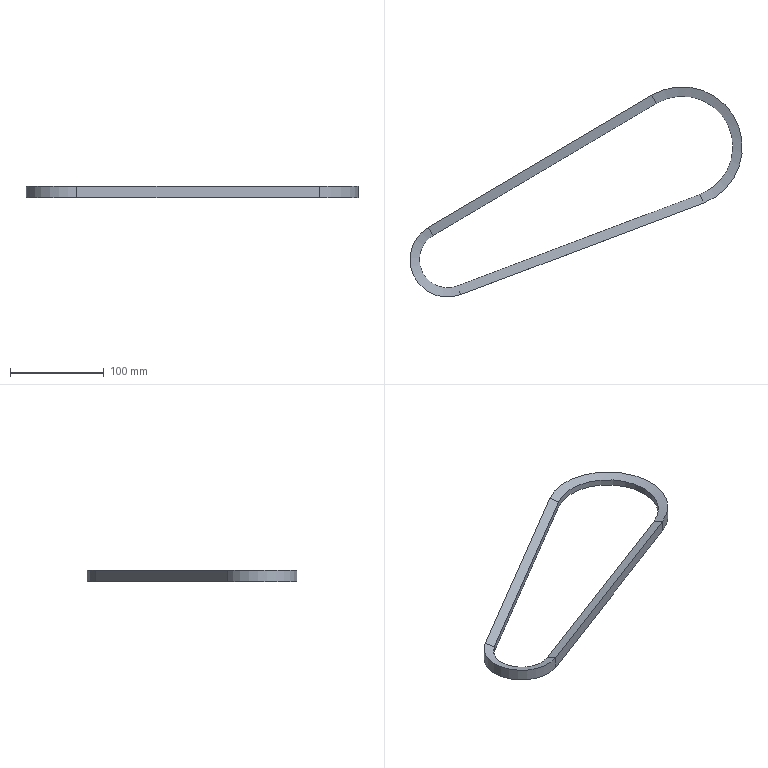Part | STEP file | Type A V-belt | 1 solid | 16 faces | box 354 x 224 x 12.68 mm | volume 82452 mm3 | plane 8 | cylinder 4 | cone 4 | commonest cylinder face diameters 60 x1 80 x1 108 x1 128 x1
STEP:
#1=CARTESIAN_POINT('',(0.,0.,0.));
#2=DIRECTION('',(0.,0.,1.));
#3=DIRECTION('',(1.,0.,0.));
#4=AXIS2_PLACEMENT_3D('',#1,#2,#3);
#5=CARTESIAN_POINT('',(10.593,-28.068,3.3));
#6=VERTEX_POINT('',#5);
#7=CARTESIAN_POINT('',(-15.274,25.821,3.3));
#8=VERTEX_POINT('',#7);
#9=CARTESIAN_POINT('',(0.,0.,3.3));
#10=DIRECTION('',(0.,0.,-1.));
#11=DIRECTION('',(-1.,0.,0.));
#12=AXIS2_PLACEMENT_3D('',#9,#10,#11);
#13=CIRCLE('',#12,30.);
#14=CARTESIAN_POINT('',(0.,0.,0.));
#15=DIRECTION('',(0.,0.,-1.));
#16=DIRECTION('',(-1.,0.,0.));
#17=AXIS2_PLACEMENT_3D('',#14,#15,#16);
#18=CYLINDRICAL_SURFACE('',#17,30.);
#19=CARTESIAN_POINT('',(0.,-3.3));
#20=DIRECTION('',(1.,0.));
#21=VECTOR('',#20,1.);
#22=LINE('',#19,#21);
#23=(GEOMETRIC_REPRESENTATION_CONTEXT(2)PARAMETRIC_REPRESENTATION_CONTEXT()REPRESENTATION_CONTEXT('',''));
#24=DEFINITIONAL_REPRESENTATION('',(#22),#23);
#25=PCURVE('',#18,#24);
#26=CARTESIAN_POINT('',(0.,0.,6.34));
#27=DIRECTION('',(0.,0.,1.));
#28=DIRECTION('',(1.,0.,0.));
#29=AXIS2_PLACEMENT_3D('',#26,#27,#28);
#30=CONICAL_SURFACE('',#29,40.,1.276);
#31=CARTESIAN_POINT('',(9.425,-3.04));
#32=DIRECTION('',(-1.,0.));
#33=VECTOR('',#32,1.);
#34=LINE('',#31,#33);
#35=(GEOMETRIC_REPRESENTATION_CONTEXT(2)PARAMETRIC_REPRESENTATION_CONTEXT()REPRESENTATION_CONTEXT('',''));
#36=DEFINITIONAL_REPRESENTATION('',(#34),#35);
#37=PCURVE('',#30,#36);
#38=SURFACE_CURVE('',#13,(#25,#37),.PCURVE_S1.);
#39=EDGE_CURVE('',#6,#8,#38,.T.);
#40=ORIENTED_EDGE('',*,*,#39,.T.);
#41=CARTESIAN_POINT('',(-15.274,25.821,-3.3));
#42=VERTEX_POINT('',#41);
#43=CARTESIAN_POINT('',(-15.274,25.821,3.3));
#44=CARTESIAN_POINT('',(-15.274,25.821,1.1));
#45=CARTESIAN_POINT('',(-15.274,25.821,-1.1));
#46=CARTESIAN_POINT('',(-15.274,25.821,-3.3));
#47=B_SPLINE_CURVE_WITH_KNOTS('',3,(#43,#44,#45,#46),.UNSPECIFIED.,.F.,.F.,(4,4),(0.,1.),.PIECEWISE_BEZIER_KNOTS.);
#48=CARTESIAN_POINT('',(7.32,-3.3));
#49=CARTESIAN_POINT('',(7.32,3.3));
#50=B_SPLINE_CURVE_WITH_KNOTS('',1,(#48,#49),.UNSPECIFIED.,.F.,.F.,(2,2),(0.,1.),.PIECEWISE_BEZIER_KNOTS.);
#51=(GEOMETRIC_REPRESENTATION_CONTEXT(2)PARAMETRIC_REPRESENTATION_CONTEXT()REPRESENTATION_CONTEXT('',''));
#52=DEFINITIONAL_REPRESENTATION('',(#50),#51);
#53=PCURVE('',#18,#52);
#54=CARTESIAN_POINT('',(222.507,166.477,-3.3));
#55=DIRECTION('',(-0.5091,0.8607,0.));
#56=DIRECTION('',(-0.8607,-0.5091,0.));
#57=AXIS2_PLACEMENT_3D('',#54,#55,#56);
#58=PLANE('',#57);
#59=CARTESIAN_POINT('',(276.268,6.6));
#60=CARTESIAN_POINT('',(276.268,4.4));
#61=CARTESIAN_POINT('',(276.268,2.2));
#62=CARTESIAN_POINT('',(276.268,0.));
#63=B_SPLINE_CURVE_WITH_KNOTS('',3,(#59,#60,#61,#62),.UNSPECIFIED.,.F.,.F.,(4,4),(0.,1.),.PIECEWISE_BEZIER_KNOTS.);
#64=(GEOMETRIC_REPRESENTATION_CONTEXT(2)PARAMETRIC_REPRESENTATION_CONTEXT()REPRESENTATION_CONTEXT('',''));
#65=DEFINITIONAL_REPRESENTATION('',(#63),#64);
#66=PCURVE('',#58,#65);
#67=SURFACE_CURVE('',#47,(#53,#66),.PCURVE_S1.);
#68=EDGE_CURVE('',#8,#42,#67,.T.);
#69=ORIENTED_EDGE('',*,*,#68,.T.);
#70=CARTESIAN_POINT('',(10.593,-28.068,-3.3));
#71=VERTEX_POINT('',#70);
#72=CARTESIAN_POINT('',(0.,0.,-3.3));
#73=DIRECTION('',(0.,0.,-1.));
#74=DIRECTION('',(-1.,0.,0.));
#75=AXIS2_PLACEMENT_3D('',#72,#73,#74);
#76=CIRCLE('',#75,30.);
#77=CARTESIAN_POINT('',(0.,3.3));
#78=DIRECTION('',(1.,0.));
#79=VECTOR('',#78,1.);
#80=LINE('',#77,#79);
#81=(GEOMETRIC_REPRESENTATION_CONTEXT(2)PARAMETRIC_REPRESENTATION_CONTEXT()REPRESENTATION_CONTEXT('',''));
#82=DEFINITIONAL_REPRESENTATION('',(#80),#81);
#83=PCURVE('',#18,#82);
#84=CARTESIAN_POINT('',(0.,0.,-3.3));
#85=DIRECTION('',(0.,0.,-1.));
#86=DIRECTION('',(-1.,0.,0.));
#87=AXIS2_PLACEMENT_3D('',#84,#85,#86);
#88=CONICAL_SURFACE('',#87,30.,1.276);
#89=CARTESIAN_POINT('',(0.,0.));
#90=DIRECTION('',(1.,0.));
#91=VECTOR('',#90,1.);
#92=LINE('',#89,#91);
#93=(GEOMETRIC_REPRESENTATION_CONTEXT(2)PARAMETRIC_REPRESENTATION_CONTEXT()REPRESENTATION_CONTEXT('',''));
#94=DEFINITIONAL_REPRESENTATION('',(#92),#93);
#95=PCURVE('',#88,#94);
#96=SURFACE_CURVE('',#76,(#83,#95),.PCURVE_S1.);
#97=EDGE_CURVE('',#71,#42,#96,.T.);
#98=ORIENTED_EDGE('',*,*,#97,.F.);
#99=CARTESIAN_POINT('',(10.593,-28.068,-3.3));
#100=DIRECTION('',(0.,0.,-1.));
#101=VECTOR('',#100,1.);
#102=LINE('',#99,#101);
#103=CARTESIAN_POINT('',(4.352,3.3));
#104=DIRECTION('',(0.,1.));
#105=VECTOR('',#104,1.);
#106=LINE('',#103,#105);
#107=(GEOMETRIC_REPRESENTATION_CONTEXT(2)PARAMETRIC_REPRESENTATION_CONTEXT()REPRESENTATION_CONTEXT('',''));
#108=DEFINITIONAL_REPRESENTATION('',(#106),#107);
#109=PCURVE('',#18,#108);
#110=CARTESIAN_POINT('',(269.067,69.478,-3.3));
#111=DIRECTION('',(-0.3531,0.9356,0.));
#112=DIRECTION('',(-0.9356,-0.3531,0.));
#113=AXIS2_PLACEMENT_3D('',#110,#111,#112);
#114=PLANE('',#113);
#115=CARTESIAN_POINT('',(276.268,0.));
#116=DIRECTION('',(0.,-1.));
#117=VECTOR('',#116,1.);
#118=LINE('',#115,#117);
#119=(GEOMETRIC_REPRESENTATION_CONTEXT(2)PARAMETRIC_REPRESENTATION_CONTEXT()REPRESENTATION_CONTEXT('',''));
#120=DEFINITIONAL_REPRESENTATION('',(#118),#119);
#121=PCURVE('',#114,#120);
#122=SURFACE_CURVE('',#102,(#109,#121),.PCURVE_S1.);
#123=EDGE_CURVE('',#6,#71,#122,.T.);
#124=ORIENTED_EDGE('',*,*,#123,.F.);
#125=EDGE_LOOP('',(#40,#69,#98,#124));
#126=FACE_BOUND('',#125,.F.);
#127=ADVANCED_FACE('',(#126),#18,.F.);
#128=ORIENTED_EDGE('',*,*,#97,.T.);
#129=CARTESIAN_POINT('',(-20.365,34.428,-6.34));
#130=VERTEX_POINT('',#129);
#131=CARTESIAN_POINT('',(-15.274,25.821,-3.3));
#132=CARTESIAN_POINT('',(-16.971,28.69,-4.313));
#133=CARTESIAN_POINT('',(-18.668,31.559,-5.327));
#134=CARTESIAN_POINT('',(-20.365,34.428,-6.34));
#135=B_SPLINE_CURVE_WITH_KNOTS('',3,(#131,#132,#133,#134),.UNSPECIFIED.,.F.,.F.,(4,4),(0.,1.),.PIECEWISE_BEZIER_KNOTS.);
#136=CARTESIAN_POINT('',(7.32,0.));
#137=CARTESIAN_POINT('',(7.32,3.04));
#138=B_SPLINE_CURVE_WITH_KNOTS('',1,(#136,#137),.UNSPECIFIED.,.F.,.F.,(2,2),(0.,1.),.PIECEWISE_BEZIER_KNOTS.);
#139=(GEOMETRIC_REPRESENTATION_CONTEXT(2)PARAMETRIC_REPRESENTATION_CONTEXT()REPRESENTATION_CONTEXT('',''));
#140=DEFINITIONAL_REPRESENTATION('',(#138),#139);
#141=PCURVE('',#88,#140);
#142=CARTESIAN_POINT('',(217.416,175.084,-6.34));
#143=DIRECTION('',(-0.1481,0.2503,0.9568));
#144=DIRECTION('',(0.,-0.9674,0.2531));
#145=AXIS2_PLACEMENT_3D('',#142,#143,#144);
#146=PLANE('',#145);
#147=CARTESIAN_POINT('',(145.172,-235.284));
#148=CARTESIAN_POINT('',(142.14,-237.));
#149=CARTESIAN_POINT('',(139.108,-238.716));
#150=CARTESIAN_POINT('',(136.076,-240.432));
#151=B_SPLINE_CURVE_WITH_KNOTS('',3,(#147,#148,#149,#150),.UNSPECIFIED.,.F.,.F.,(4,4),(0.,1.),.PIECEWISE_BEZIER_KNOTS.);
#152=(GEOMETRIC_REPRESENTATION_CONTEXT(2)PARAMETRIC_REPRESENTATION_CONTEXT()REPRESENTATION_CONTEXT('',''));
#153=DEFINITIONAL_REPRESENTATION('',(#151),#152);
#154=PCURVE('',#146,#153);
#155=SURFACE_CURVE('',#135,(#141,#154),.PCURVE_S1.);
#156=EDGE_CURVE('',#42,#130,#155,.T.);
#157=ORIENTED_EDGE('',*,*,#156,.T.);
#158=CARTESIAN_POINT('',(14.123,-37.424,-6.34));
#159=VERTEX_POINT('',#158);
#160=CARTESIAN_POINT('',(0.,0.,-6.34));
#161=DIRECTION('',(0.,0.,-1.));
#162=DIRECTION('',(-1.,0.,0.));
#163=AXIS2_PLACEMENT_3D('',#160,#161,#162);
#164=CIRCLE('',#163,40.);
#165=CARTESIAN_POINT('',(0.,3.04));
#166=DIRECTION('',(1.,0.));
#167=VECTOR('',#166,1.);
#168=LINE('',#165,#167);
#169=(GEOMETRIC_REPRESENTATION_CONTEXT(2)PARAMETRIC_REPRESENTATION_CONTEXT()REPRESENTATION_CONTEXT('',''));
#170=DEFINITIONAL_REPRESENTATION('',(#168),#169);
#171=PCURVE('',#88,#170);
#172=CARTESIAN_POINT('',(0.,0.,0.));
#173=DIRECTION('',(0.,0.,-1.));
#174=DIRECTION('',(-1.,0.,0.));
#175=AXIS2_PLACEMENT_3D('',#172,#173,#174);
#176=CYLINDRICAL_SURFACE('',#175,40.);
#177=CARTESIAN_POINT('',(0.,6.34));
#178=DIRECTION('',(1.,0.));
#179=VECTOR('',#178,1.);
#180=LINE('',#177,#179);
#181=(GEOMETRIC_REPRESENTATION_CONTEXT(2)PARAMETRIC_REPRESENTATION_CONTEXT()REPRESENTATION_CONTEXT('',''));
#182=DEFINITIONAL_REPRESENTATION('',(#180),#181);
#183=PCURVE('',#176,#182);
#184=SURFACE_CURVE('',#164,(#171,#183),.PCURVE_S1.);
#185=EDGE_CURVE('',#159,#130,#184,.T.);
#186=ORIENTED_EDGE('',*,*,#185,.F.);
#187=CARTESIAN_POINT('',(14.123,-37.424,-6.34));
#188=DIRECTION('',(0.3378,-0.8951,-0.2909));
#189=VECTOR('',#188,1.);
#190=LINE('',#187,#189);
#191=CARTESIAN_POINT('',(4.352,3.04));
#192=DIRECTION('',(0.,1.));
#193=VECTOR('',#192,1.);
#194=LINE('',#191,#193);
#195=(GEOMETRIC_REPRESENTATION_CONTEXT(2)PARAMETRIC_REPRESENTATION_CONTEXT()REPRESENTATION_CONTEXT('',''));
#196=DEFINITIONAL_REPRESENTATION('',(#194),#195);
#197=PCURVE('',#88,#196);
#198=CARTESIAN_POINT('',(272.597,60.122,-6.34));
#199=DIRECTION('',(-0.1027,0.2721,-0.9568));
#200=DIRECTION('',(0.,0.9619,0.2736));
#201=AXIS2_PLACEMENT_3D('',#198,#199,#200);
#202=PLANE('',#201);
#203=CARTESIAN_POINT('',(-93.825,-259.848));
#204=DIRECTION('',(-0.9406,0.3396));
#205=VECTOR('',#204,1.);
#206=LINE('',#203,#205);
#207=(GEOMETRIC_REPRESENTATION_CONTEXT(2)PARAMETRIC_REPRESENTATION_CONTEXT()REPRESENTATION_CONTEXT('',''));
#208=DEFINITIONAL_REPRESENTATION('',(#206),#207);
#209=PCURVE('',#202,#208);
#210=SURFACE_CURVE('',#190,(#197,#209),.PCURVE_S1.);
#211=EDGE_CURVE('',#71,#159,#210,.T.);
#212=ORIENTED_EDGE('',*,*,#211,.F.);
#213=EDGE_LOOP('',(#128,#157,#186,#212));
#214=FACE_BOUND('',#213,.F.);
#215=ADVANCED_FACE('',(#214),#88,.F.);
#216=CARTESIAN_POINT('',(14.123,-37.424,6.34));
#217=VERTEX_POINT('',#216);
#218=CARTESIAN_POINT('',(14.123,-37.424,6.34));
#219=DIRECTION('',(0.,0.,1.));
#220=VECTOR('',#219,1.);
#221=LINE('',#218,#220);
#222=CARTESIAN_POINT('',(4.352,-6.34));
#223=DIRECTION('',(0.,-1.));
#224=VECTOR('',#223,1.);
#225=LINE('',#222,#224);
#226=(GEOMETRIC_REPRESENTATION_CONTEXT(2)PARAMETRIC_REPRESENTATION_CONTEXT()REPRESENTATION_CONTEXT('',''));
#227=DEFINITIONAL_REPRESENTATION('',(#225),#226);
#228=PCURVE('',#176,#227);
#229=CARTESIAN_POINT('',(272.597,60.122,6.34));
#230=DIRECTION('',(0.3531,-0.9356,0.));
#231=DIRECTION('',(0.9356,0.3531,0.));
#232=AXIS2_PLACEMENT_3D('',#229,#230,#231);
#233=PLANE('',#232);
#234=CARTESIAN_POINT('',(-276.268,0.));
#235=DIRECTION('',(0.,1.));
#236=VECTOR('',#235,1.);
#237=LINE('',#234,#236);
#238=(GEOMETRIC_REPRESENTATION_CONTEXT(2)PARAMETRIC_REPRESENTATION_CONTEXT()REPRESENTATION_CONTEXT('',''));
#239=DEFINITIONAL_REPRESENTATION('',(#237),#238);
#240=PCURVE('',#233,#239);
#241=SURFACE_CURVE('',#221,(#228,#240),.PCURVE_S1.);
#242=EDGE_CURVE('',#159,#217,#241,.T.);
#243=ORIENTED_EDGE('',*,*,#242,.T.);
#244=CARTESIAN_POINT('',(-20.365,34.428,6.34));
#245=VERTEX_POINT('',#244);
#246=CARTESIAN_POINT('',(0.,0.,6.34));
#247=DIRECTION('',(0.,0.,-1.));
#248=DIRECTION('',(-1.,0.,0.));
#249=AXIS2_PLACEMENT_3D('',#246,#247,#248);
#250=CIRCLE('',#249,40.);
#251=CARTESIAN_POINT('',(0.,-6.34));
#252=DIRECTION('',(1.,0.));
#253=VECTOR('',#252,1.);
#254=LINE('',#251,#253);
#255=(GEOMETRIC_REPRESENTATION_CONTEXT(2)PARAMETRIC_REPRESENTATION_CONTEXT()REPRESENTATION_CONTEXT('',''));
#256=DEFINITIONAL_REPRESENTATION('',(#254),#255);
#257=PCURVE('',#176,#256);
#258=CARTESIAN_POINT('',(9.425,0.));
#259=DIRECTION('',(-1.,0.));
#260=VECTOR('',#259,1.);
#261=LINE('',#258,#260);
#262=(GEOMETRIC_REPRESENTATION_CONTEXT(2)PARAMETRIC_REPRESENTATION_CONTEXT()REPRESENTATION_CONTEXT('',''));
#263=DEFINITIONAL_REPRESENTATION('',(#261),#262);
#264=PCURVE('',#30,#263);
#265=SURFACE_CURVE('',#250,(#257,#264),.PCURVE_S1.);
#266=EDGE_CURVE('',#217,#245,#265,.T.);
#267=ORIENTED_EDGE('',*,*,#266,.T.);
#268=CARTESIAN_POINT('',(-20.365,34.428,-6.34));
#269=CARTESIAN_POINT('',(-20.365,34.428,-2.113));
#270=CARTESIAN_POINT('',(-20.365,34.428,2.113));
#271=CARTESIAN_POINT('',(-20.365,34.428,6.34));
#272=B_SPLINE_CURVE_WITH_KNOTS('',3,(#268,#269,#270,#271),.UNSPECIFIED.,.F.,.F.,(4,4),(0.,1.),.PIECEWISE_BEZIER_KNOTS.);
#273=CARTESIAN_POINT('',(7.32,6.34));
#274=CARTESIAN_POINT('',(7.32,-6.34));
#275=B_SPLINE_CURVE_WITH_KNOTS('',1,(#273,#274),.UNSPECIFIED.,.F.,.F.,(2,2),(0.,1.),.PIECEWISE_BEZIER_KNOTS.);
#276=(GEOMETRIC_REPRESENTATION_CONTEXT(2)PARAMETRIC_REPRESENTATION_CONTEXT()REPRESENTATION_CONTEXT('',''));
#277=DEFINITIONAL_REPRESENTATION('',(#275),#276);
#278=PCURVE('',#176,#277);
#279=CARTESIAN_POINT('',(217.416,175.084,6.34));
#280=DIRECTION('',(0.5091,-0.8607,0.));
#281=DIRECTION('',(0.8607,0.5091,0.));
#282=AXIS2_PLACEMENT_3D('',#279,#280,#281);
#283=PLANE('',#282);
#284=CARTESIAN_POINT('',(-276.268,-12.68));
#285=CARTESIAN_POINT('',(-276.268,-8.453));
#286=CARTESIAN_POINT('',(-276.268,-4.227));
#287=CARTESIAN_POINT('',(-276.268,0.));
#288=B_SPLINE_CURVE_WITH_KNOTS('',3,(#284,#285,#286,#287),.UNSPECIFIED.,.F.,.F.,(4,4),(0.,1.),.PIECEWISE_BEZIER_KNOTS.);
#289=(GEOMETRIC_REPRESENTATION_CONTEXT(2)PARAMETRIC_REPRESENTATION_CONTEXT()REPRESENTATION_CONTEXT('',''));
#290=DEFINITIONAL_REPRESENTATION('',(#288),#289);
#291=PCURVE('',#283,#290);
#292=SURFACE_CURVE('',#272,(#278,#291),.PCURVE_S1.);
#293=EDGE_CURVE('',#130,#245,#292,.T.);
#294=ORIENTED_EDGE('',*,*,#293,.F.);
#295=ORIENTED_EDGE('',*,*,#185,.F.);
#296=EDGE_LOOP('',(#243,#267,#294,#295));
#297=FACE_BOUND('',#296,.T.);
#298=ADVANCED_FACE('',(#297),#176,.T.);
#299=ORIENTED_EDGE('',*,*,#266,.T.);
#300=CARTESIAN_POINT('',(-20.365,34.428,6.34));
#301=CARTESIAN_POINT('',(-18.668,31.559,5.327));
#302=CARTESIAN_POINT('',(-16.971,28.69,4.313));
#303=CARTESIAN_POINT('',(-15.274,25.821,3.3));
#304=B_SPLINE_CURVE_WITH_KNOTS('',3,(#300,#301,#302,#303),.UNSPECIFIED.,.F.,.F.,(4,4),(0.,1.),.PIECEWISE_BEZIER_KNOTS.);
#305=CARTESIAN_POINT('',(2.105,0.));
#306=CARTESIAN_POINT('',(2.105,-3.04));
#307=B_SPLINE_CURVE_WITH_KNOTS('',1,(#305,#306),.UNSPECIFIED.,.F.,.F.,(2,2),(0.,1.),.PIECEWISE_BEZIER_KNOTS.);
#308=(GEOMETRIC_REPRESENTATION_CONTEXT(2)PARAMETRIC_REPRESENTATION_CONTEXT()REPRESENTATION_CONTEXT('',''));
#309=DEFINITIONAL_REPRESENTATION('',(#307),#308);
#310=PCURVE('',#30,#309);
#311=CARTESIAN_POINT('',(222.507,166.477,3.3));
#312=DIRECTION('',(-0.1481,0.2503,-0.9568));
#313=DIRECTION('',(0.,0.9674,0.2531));
#314=AXIS2_PLACEMENT_3D('',#311,#312,#313);
#315=PLANE('',#314);
#316=CARTESIAN_POINT('',(-126.98,-245.58));
#317=CARTESIAN_POINT('',(-130.012,-243.864));
#318=CARTESIAN_POINT('',(-133.044,-242.148));
#319=CARTESIAN_POINT('',(-136.076,-240.432));
#320=B_SPLINE_CURVE_WITH_KNOTS('',3,(#316,#317,#318,#319),.UNSPECIFIED.,.F.,.F.,(4,4),(0.,1.),.PIECEWISE_BEZIER_KNOTS.);
#321=(GEOMETRIC_REPRESENTATION_CONTEXT(2)PARAMETRIC_REPRESENTATION_CONTEXT()REPRESENTATION_CONTEXT('',''));
#322=DEFINITIONAL_REPRESENTATION('',(#320),#321);
#323=PCURVE('',#315,#322);
#324=SURFACE_CURVE('',#304,(#310,#323),.PCURVE_S1.);
#325=EDGE_CURVE('',#245,#8,#324,.T.);
#326=ORIENTED_EDGE('',*,*,#325,.T.);
#327=ORIENTED_EDGE('',*,*,#39,.F.);
#328=CARTESIAN_POINT('',(10.593,-28.068,3.3));
#329=DIRECTION('',(-0.3378,0.8951,-0.2909));
#330=VECTOR('',#329,1.);
#331=LINE('',#328,#330);
#332=CARTESIAN_POINT('',(5.073,-3.04));
#333=DIRECTION('',(0.,-1.));
#334=VECTOR('',#333,1.);
#335=LINE('',#332,#334);
#336=(GEOMETRIC_REPRESENTATION_CONTEXT(2)PARAMETRIC_REPRESENTATION_CONTEXT()REPRESENTATION_CONTEXT('',''));
#337=DEFINITIONAL_REPRESENTATION('',(#335),#336);
#338=PCURVE('',#30,#337);
#339=CARTESIAN_POINT('',(269.067,69.478,3.3));
#340=DIRECTION('',(-0.1027,0.2721,0.9568));
#341=DIRECTION('',(0.,-0.9619,0.2736));
#342=AXIS2_PLACEMENT_3D('',#339,#340,#341);
#343=PLANE('',#342);
#344=CARTESIAN_POINT('',(93.825,-259.848));
#345=DIRECTION('',(-0.9406,-0.3396));
#346=VECTOR('',#345,1.);
#347=LINE('',#344,#346);
#348=(GEOMETRIC_REPRESENTATION_CONTEXT(2)PARAMETRIC_REPRESENTATION_CONTEXT()REPRESENTATION_CONTEXT('',''));
#349=DEFINITIONAL_REPRESENTATION('',(#347),#348);
#350=PCURVE('',#343,#349);
#351=SURFACE_CURVE('',#331,(#338,#350),.PCURVE_S1.);
#352=EDGE_CURVE('',#217,#6,#351,.T.);
#353=ORIENTED_EDGE('',*,*,#352,.F.);
#354=EDGE_LOOP('',(#299,#326,#327,#353));
#355=FACE_BOUND('',#354,.F.);
#356=ADVANCED_FACE('',(#355),#30,.F.);
#357=CARTESIAN_POINT('',(269.067,69.478,3.3));
#358=VERTEX_POINT('',#357);
#359=CARTESIAN_POINT('',(269.067,69.478,-3.3));
#360=VERTEX_POINT('',#359);
#361=CARTESIAN_POINT('',(269.067,69.478,-3.3));
#362=DIRECTION('',(0.,0.,-1.));
#363=VECTOR('',#362,1.);
#364=LINE('',#361,#363);
#365=CARTESIAN_POINT('',(0.,0.));
#366=DIRECTION('',(0.,-1.));
#367=VECTOR('',#366,1.);
#368=LINE('',#365,#367);
#369=(GEOMETRIC_REPRESENTATION_CONTEXT(2)PARAMETRIC_REPRESENTATION_CONTEXT()REPRESENTATION_CONTEXT('',''));
#370=DEFINITIONAL_REPRESENTATION('',(#368),#369);
#371=PCURVE('',#114,#370);
#372=CARTESIAN_POINT('',(250.,120.,0.));
#373=DIRECTION('',(0.,0.,-1.));
#374=DIRECTION('',(-1.,0.,0.));
#375=AXIS2_PLACEMENT_3D('',#372,#373,#374);
#376=CYLINDRICAL_SURFACE('',#375,54.);
#377=CARTESIAN_POINT('',(4.352,3.3));
#378=DIRECTION('',(0.,1.));
#379=VECTOR('',#378,1.);
#380=LINE('',#377,#379);
#381=(GEOMETRIC_REPRESENTATION_CONTEXT(2)PARAMETRIC_REPRESENTATION_CONTEXT()REPRESENTATION_CONTEXT('',''));
#382=DEFINITIONAL_REPRESENTATION('',(#380),#381);
#383=PCURVE('',#376,#382);
#384=SURFACE_CURVE('',#364,(#371,#383),.PCURVE_S1.);
#385=EDGE_CURVE('',#358,#360,#384,.T.);
#386=ORIENTED_EDGE('',*,*,#385,.T.);
#387=CARTESIAN_POINT('',(269.067,69.478,-3.3));
#388=DIRECTION('',(-0.9356,-0.3531,0.));
#389=VECTOR('',#388,1.);
#390=LINE('',#387,#389);
#391=CARTESIAN_POINT('',(0.,0.));
#392=DIRECTION('',(1.,0.));
#393=VECTOR('',#392,1.);
#394=LINE('',#391,#393);
#395=(GEOMETRIC_REPRESENTATION_CONTEXT(2)PARAMETRIC_REPRESENTATION_CONTEXT()REPRESENTATION_CONTEXT('',''));
#396=DEFINITIONAL_REPRESENTATION('',(#394),#395);
#397=PCURVE('',#114,#396);
#398=CARTESIAN_POINT('',(9.831,-3.55));
#399=DIRECTION('',(-0.3396,-0.9406));
#400=VECTOR('',#399,1.);
#401=LINE('',#398,#400);
#402=(GEOMETRIC_REPRESENTATION_CONTEXT(2)PARAMETRIC_REPRESENTATION_CONTEXT()REPRESENTATION_CONTEXT('',''));
#403=DEFINITIONAL_REPRESENTATION('',(#401),#402);
#404=PCURVE('',#202,#403);
#405=SURFACE_CURVE('',#390,(#397,#404),.PCURVE_S1.);
#406=EDGE_CURVE('',#360,#71,#405,.T.);
#407=ORIENTED_EDGE('',*,*,#406,.T.);
#408=ORIENTED_EDGE('',*,*,#123,.F.);
#409=CARTESIAN_POINT('',(269.067,69.478,3.3));
#410=DIRECTION('',(-0.9356,-0.3531,0.));
#411=VECTOR('',#410,1.);
#412=LINE('',#409,#411);
#413=CARTESIAN_POINT('',(0.,6.6));
#414=DIRECTION('',(1.,0.));
#415=VECTOR('',#414,1.);
#416=LINE('',#413,#415);
#417=(GEOMETRIC_REPRESENTATION_CONTEXT(2)PARAMETRIC_REPRESENTATION_CONTEXT()REPRESENTATION_CONTEXT('',''));
#418=DEFINITIONAL_REPRESENTATION('',(#416),#417);
#419=PCURVE('',#114,#418);
#420=CARTESIAN_POINT('',(0.,0.));
#421=DIRECTION('',(0.3396,-0.9406));
#422=VECTOR('',#421,1.);
#423=LINE('',#420,#422);
#424=(GEOMETRIC_REPRESENTATION_CONTEXT(2)PARAMETRIC_REPRESENTATION_CONTEXT()REPRESENTATION_CONTEXT('',''));
#425=DEFINITIONAL_REPRESENTATION('',(#423),#424);
#426=PCURVE('',#343,#425);
#427=SURFACE_CURVE('',#412,(#419,#426),.PCURVE_S1.);
#428=EDGE_CURVE('',#358,#6,#427,.T.);
#429=ORIENTED_EDGE('',*,*,#428,.F.);
#430=EDGE_LOOP('',(#386,#407,#408,#429));
#431=FACE_BOUND('',#430,.T.);
#432=ADVANCED_FACE('',(#431),#114,.T.);
#433=CARTESIAN_POINT('',(272.597,60.122,-6.34));
#434=VERTEX_POINT('',#433);
#435=CARTESIAN_POINT('',(272.597,60.122,-6.34));
#436=DIRECTION('',(0.3378,-0.8951,-0.2909));
#437=VECTOR('',#436,1.);
#438=LINE('',#435,#437);
#439=CARTESIAN_POINT('',(0.,0.));
#440=DIRECTION('',(-0.9406,0.3396));
#441=VECTOR('',#440,1.);
#442=LINE('',#439,#441);
#443=(GEOMETRIC_REPRESENTATION_CONTEXT(2)PARAMETRIC_REPRESENTATION_CONTEXT()REPRESENTATION_CONTEXT('',''));
#444=DEFINITIONAL_REPRESENTATION('',(#442),#443);
#445=PCURVE('',#202,#444);
#446=CARTESIAN_POINT('',(250.,120.,-3.3));
#447=DIRECTION('',(0.,0.,-1.));
#448=DIRECTION('',(-1.,0.,0.));
#449=AXIS2_PLACEMENT_3D('',#446,#447,#448);
#450=CONICAL_SURFACE('',#449,54.,1.276);
#451=CARTESIAN_POINT('',(4.352,3.04));
#452=DIRECTION('',(0.,1.));
#453=VECTOR('',#452,1.);
#454=LINE('',#451,#453);
#455=(GEOMETRIC_REPRESENTATION_CONTEXT(2)PARAMETRIC_REPRESENTATION_CONTEXT()REPRESENTATION_CONTEXT('',''));
#456=DEFINITIONAL_REPRESENTATION('',(#454),#455);
#457=PCURVE('',#450,#456);
#458=SURFACE_CURVE('',#438,(#445,#457),.PCURVE_S1.);
#459=EDGE_CURVE('',#360,#434,#458,.T.);
#460=ORIENTED_EDGE('',*,*,#459,.T.);
#461=CARTESIAN_POINT('',(272.597,60.122,-6.34));
#462=DIRECTION('',(-0.9356,-0.3531,0.));
#463=VECTOR('',#462,1.);
#464=LINE('',#461,#463);
#465=CARTESIAN_POINT('',(0.,0.));
#466=DIRECTION('',(-0.3396,-0.9406));
#467=VECTOR('',#466,1.);
#468=LINE('',#465,#467);
#469=(GEOMETRIC_REPRESENTATION_CONTEXT(2)PARAMETRIC_REPRESENTATION_CONTEXT()REPRESENTATION_CONTEXT('',''));
#470=DEFINITIONAL_REPRESENTATION('',(#468),#469);
#471=PCURVE('',#202,#470);
#472=CARTESIAN_POINT('',(0.,-12.68));
#473=DIRECTION('',(-1.,0.));
#474=VECTOR('',#473,1.);
#475=LINE('',#472,#474);
#476=(GEOMETRIC_REPRESENTATION_CONTEXT(2)PARAMETRIC_REPRESENTATION_CONTEXT()REPRESENTATION_CONTEXT('',''));
#477=DEFINITIONAL_REPRESENTATION('',(#475),#476);
#478=PCURVE('',#233,#477);
#479=SURFACE_CURVE('',#464,(#471,#478),.PCURVE_S1.);
#480=EDGE_CURVE('',#434,#159,#479,.T.);
#481=ORIENTED_EDGE('',*,*,#480,.T.);
#482=ORIENTED_EDGE('',*,*,#211,.F.);
#483=ORIENTED_EDGE('',*,*,#406,.F.);
#484=EDGE_LOOP('',(#460,#481,#482,#483));
#485=FACE_BOUND('',#484,.T.);
#486=ADVANCED_FACE('',(#485),#202,.T.);
#487=CARTESIAN_POINT('',(272.597,60.122,6.34));
#488=VERTEX_POINT('',#487);
#489=CARTESIAN_POINT('',(272.597,60.122,6.34));
#490=DIRECTION('',(0.,0.,1.));
#491=VECTOR('',#490,1.);
#492=LINE('',#489,#491);
#493=CARTESIAN_POINT('',(0.,0.));
#494=DIRECTION('',(0.,1.));
#495=VECTOR('',#494,1.);
#496=LINE('',#493,#495);
#497=(GEOMETRIC_REPRESENTATION_CONTEXT(2)PARAMETRIC_REPRESENTATION_CONTEXT()REPRESENTATION_CONTEXT('',''));
#498=DEFINITIONAL_REPRESENTATION('',(#496),#497);
#499=PCURVE('',#233,#498);
#500=CARTESIAN_POINT('',(250.,120.,0.));
#501=DIRECTION('',(0.,0.,-1.));
#502=DIRECTION('',(-1.,0.,0.));
#503=AXIS2_PLACEMENT_3D('',#500,#501,#502);
#504=CYLINDRICAL_SURFACE('',#503,64.);
#505=CARTESIAN_POINT('',(4.352,-6.34));
#506=DIRECTION('',(0.,-1.));
#507=VECTOR('',#506,1.);
#508=LINE('',#505,#507);
#509=(GEOMETRIC_REPRESENTATION_CONTEXT(2)PARAMETRIC_REPRESENTATION_CONTEXT()REPRESENTATION_CONTEXT('',''));
#510=DEFINITIONAL_REPRESENTATION('',(#508),#509);
#511=PCURVE('',#504,#510);
#512=SURFACE_CURVE('',#492,(#499,#511),.PCURVE_S1.);
#513=EDGE_CURVE('',#434,#488,#512,.T.);
#514=ORIENTED_EDGE('',*,*,#513,.T.);
#515=CARTESIAN_POINT('',(272.597,60.122,6.34));
#516=DIRECTION('',(-0.9356,-0.3531,0.));
#517=VECTOR('',#516,1.);
#518=LINE('',#515,#517);
#519=CARTESIAN_POINT('',(0.,0.));
#520=DIRECTION('',(-1.,0.));
#521=VECTOR('',#520,1.);
#522=LINE('',#519,#521);
#523=(GEOMETRIC_REPRESENTATION_CONTEXT(2)PARAMETRIC_REPRESENTATION_CONTEXT()REPRESENTATION_CONTEXT('',''));
#524=DEFINITIONAL_REPRESENTATION('',(#522),#523);
#525=PCURVE('',#233,#524);
#526=CARTESIAN_POINT('',(9.831,3.55));
#527=DIRECTION('',(0.3396,-0.9406));
#528=VECTOR('',#527,1.);
#529=LINE('',#526,#528);
#530=(GEOMETRIC_REPRESENTATION_CONTEXT(2)PARAMETRIC_REPRESENTATION_CONTEXT()REPRESENTATION_CONTEXT('',''));
#531=DEFINITIONAL_REPRESENTATION('',(#529),#530);
#532=PCURVE('',#343,#531);
#533=SURFACE_CURVE('',#518,(#525,#532),.PCURVE_S1.);
#534=EDGE_CURVE('',#488,#217,#533,.T.);
#535=ORIENTED_EDGE('',*,*,#534,.T.);
#536=ORIENTED_EDGE('',*,*,#242,.F.);
#537=ORIENTED_EDGE('',*,*,#480,.F.);
#538=EDGE_LOOP('',(#514,#535,#536,#537));
#539=FACE_BOUND('',#538,.T.);
#540=ADVANCED_FACE('',(#539),#233,.T.);
#541=CARTESIAN_POINT('',(269.067,69.478,3.3));
#542=DIRECTION('',(-0.3378,0.8951,-0.2909));
#543=VECTOR('',#542,1.);
#544=LINE('',#541,#543);
#545=CARTESIAN_POINT('',(0.,0.));
#546=DIRECTION('',(-0.9406,-0.3396));
#547=VECTOR('',#546,1.);
#548=LINE('',#545,#547);
#549=(GEOMETRIC_REPRESENTATION_CONTEXT(2)PARAMETRIC_REPRESENTATION_CONTEXT()REPRESENTATION_CONTEXT('',''));
#550=DEFINITIONAL_REPRESENTATION('',(#548),#549);
#551=PCURVE('',#343,#550);
#552=CARTESIAN_POINT('',(250.,120.,6.34));
#553=DIRECTION('',(0.,0.,1.));
#554=DIRECTION('',(1.,0.,0.));
#555=AXIS2_PLACEMENT_3D('',#552,#553,#554);
#556=CONICAL_SURFACE('',#555,64.,1.276);
#557=CARTESIAN_POINT('',(-1.21,-3.04));
#558=DIRECTION('',(0.,-1.));
#559=VECTOR('',#558,1.);
#560=LINE('',#557,#559);
#561=(GEOMETRIC_REPRESENTATION_CONTEXT(2)PARAMETRIC_REPRESENTATION_CONTEXT()REPRESENTATION_CONTEXT('',''));
#562=DEFINITIONAL_REPRESENTATION('',(#560),#561);
#563=PCURVE('',#556,#562);
#564=SURFACE_CURVE('',#544,(#551,#563),.PCURVE_S1.);
#565=EDGE_CURVE('',#488,#358,#564,.T.);
#566=ORIENTED_EDGE('',*,*,#565,.T.);
#567=ORIENTED_EDGE('',*,*,#428,.T.);
#568=ORIENTED_EDGE('',*,*,#352,.F.);
#569=ORIENTED_EDGE('',*,*,#534,.F.);
#570=EDGE_LOOP('',(#566,#567,#568,#569));
#571=FACE_BOUND('',#570,.T.);
#572=ADVANCED_FACE('',(#571),#343,.T.);
#573=CARTESIAN_POINT('',(222.507,166.477,3.3));
#574=VERTEX_POINT('',#573);
#575=CARTESIAN_POINT('',(250.,120.,3.3));
#576=DIRECTION('',(0.,0.,-1.));
#577=DIRECTION('',(-1.,0.,0.));
#578=AXIS2_PLACEMENT_3D('',#575,#576,#577);
#579=CIRCLE('',#578,54.);
#580=CARTESIAN_POINT('',(0.,-3.3));
#581=DIRECTION('',(1.,0.));
#582=VECTOR('',#581,1.);
#583=LINE('',#580,#582);
#584=(GEOMETRIC_REPRESENTATION_CONTEXT(2)PARAMETRIC_REPRESENTATION_CONTEXT()REPRESENTATION_CONTEXT('',''));
#585=DEFINITIONAL_REPRESENTATION('',(#583),#584);
#586=PCURVE('',#376,#585);
#587=CARTESIAN_POINT('',(3.142,-3.04));
#588=DIRECTION('',(-1.,0.));
#589=VECTOR('',#588,1.);
#590=LINE('',#587,#589);
#591=(GEOMETRIC_REPRESENTATION_CONTEXT(2)PARAMETRIC_REPRESENTATION_CONTEXT()REPRESENTATION_CONTEXT('',''));
#592=DEFINITIONAL_REPRESENTATION('',(#590),#591);
#593=PCURVE('',#556,#592);
#594=SURFACE_CURVE('',#579,(#586,#593),.PCURVE_S1.);
#595=EDGE_CURVE('',#574,#358,#594,.T.);
#596=ORIENTED_EDGE('',*,*,#595,.T.);
#597=ORIENTED_EDGE('',*,*,#385,.T.);
#598=CARTESIAN_POINT('',(222.507,166.477,-3.3));
#599=VERTEX_POINT('',#598);
#600=CARTESIAN_POINT('',(250.,120.,-3.3));
#601=DIRECTION('',(0.,0.,-1.));
#602=DIRECTION('',(-1.,0.,0.));
#603=AXIS2_PLACEMENT_3D('',#600,#601,#602);
#604=CIRCLE('',#603,54.);
#605=CARTESIAN_POINT('',(0.,3.3));
#606=DIRECTION('',(1.,0.));
#607=VECTOR('',#606,1.);
#608=LINE('',#605,#607);
#609=(GEOMETRIC_REPRESENTATION_CONTEXT(2)PARAMETRIC_REPRESENTATION_CONTEXT()REPRESENTATION_CONTEXT('',''));
#610=DEFINITIONAL_REPRESENTATION('',(#608),#609);
#611=PCURVE('',#376,#610);
#612=CARTESIAN_POINT('',(0.,0.));
#613=DIRECTION('',(1.,0.));
#614=VECTOR('',#613,1.);
#615=LINE('',#612,#614);
#616=(GEOMETRIC_REPRESENTATION_CONTEXT(2)PARAMETRIC_REPRESENTATION_CONTEXT()REPRESENTATION_CONTEXT('',''));
#617=DEFINITIONAL_REPRESENTATION('',(#615),#616);
#618=PCURVE('',#450,#617);
#619=SURFACE_CURVE('',#604,(#611,#618),.PCURVE_S1.);
#620=EDGE_CURVE('',#599,#360,#619,.T.);
#621=ORIENTED_EDGE('',*,*,#620,.F.);
#622=CARTESIAN_POINT('',(222.507,166.477,-3.3));
#623=DIRECTION('',(0.,0.,-1.));
#624=VECTOR('',#623,1.);
#625=LINE('',#622,#624);
#626=CARTESIAN_POINT('',(1.037,3.3));
#627=DIRECTION('',(0.,1.));
#628=VECTOR('',#627,1.);
#629=LINE('',#626,#628);
#630=(GEOMETRIC_REPRESENTATION_CONTEXT(2)PARAMETRIC_REPRESENTATION_CONTEXT()REPRESENTATION_CONTEXT('',''));
#631=DEFINITIONAL_REPRESENTATION('',(#629),#630);
#632=PCURVE('',#376,#631);
#633=CARTESIAN_POINT('',(0.,0.));
#634=DIRECTION('',(0.,-1.));
#635=VECTOR('',#634,1.);
#636=LINE('',#633,#635);
#637=(GEOMETRIC_REPRESENTATION_CONTEXT(2)PARAMETRIC_REPRESENTATION_CONTEXT()REPRESENTATION_CONTEXT('',''));
#638=DEFINITIONAL_REPRESENTATION('',(#636),#637);
#639=PCURVE('',#58,#638);
#640=SURFACE_CURVE('',#625,(#632,#639),.PCURVE_S1.);
#641=EDGE_CURVE('',#574,#599,#640,.T.);
#642=ORIENTED_EDGE('',*,*,#641,.F.);
#643=EDGE_LOOP('',(#596,#597,#621,#642));
#644=FACE_BOUND('',#643,.F.);
#645=ADVANCED_FACE('',(#644),#376,.F.);
#646=ORIENTED_EDGE('',*,*,#620,.T.);
#647=ORIENTED_EDGE('',*,*,#459,.T.);
#648=CARTESIAN_POINT('',(217.416,175.084,-6.34));
#649=VERTEX_POINT('',#648);
#650=CARTESIAN_POINT('',(250.,120.,-6.34));
#651=DIRECTION('',(0.,0.,-1.));
#652=DIRECTION('',(-1.,0.,0.));
#653=AXIS2_PLACEMENT_3D('',#650,#651,#652);
#654=CIRCLE('',#653,64.);
#655=CARTESIAN_POINT('',(0.,3.04));
#656=DIRECTION('',(1.,0.));
#657=VECTOR('',#656,1.);
#658=LINE('',#655,#657);
#659=(GEOMETRIC_REPRESENTATION_CONTEXT(2)PARAMETRIC_REPRESENTATION_CONTEXT()REPRESENTATION_CONTEXT('',''));
#660=DEFINITIONAL_REPRESENTATION('',(#658),#659);
#661=PCURVE('',#450,#660);
#662=CARTESIAN_POINT('',(0.,6.34));
#663=DIRECTION('',(1.,0.));
#664=VECTOR('',#663,1.);
#665=LINE('',#662,#664);
#666=(GEOMETRIC_REPRESENTATION_CONTEXT(2)PARAMETRIC_REPRESENTATION_CONTEXT()REPRESENTATION_CONTEXT('',''));
#667=DEFINITIONAL_REPRESENTATION('',(#665),#666);
#668=PCURVE('',#504,#667);
#669=SURFACE_CURVE('',#654,(#661,#668),.PCURVE_S1.);
#670=EDGE_CURVE('',#649,#434,#669,.T.);
#671=ORIENTED_EDGE('',*,*,#670,.F.);
#672=CARTESIAN_POINT('',(217.416,175.084,-6.34));
#673=DIRECTION('',(-0.4871,0.8235,-0.2909));
#674=VECTOR('',#673,1.);
#675=LINE('',#672,#674);
#676=CARTESIAN_POINT('',(1.037,3.04));
#677=DIRECTION('',(0.,1.));
#678=VECTOR('',#677,1.);
#679=LINE('',#676,#678);
#680=(GEOMETRIC_REPRESENTATION_CONTEXT(2)PARAMETRIC_REPRESENTATION_CONTEXT()REPRESENTATION_CONTEXT('',''));
#681=DEFINITIONAL_REPRESENTATION('',(#679),#680);
#682=PCURVE('',#450,#681);
#683=CARTESIAN_POINT('',(0.,0.));
#684=DIRECTION('',(-0.8703,-0.4925));
#685=VECTOR('',#684,1.);
#686=LINE('',#683,#685);
#687=(GEOMETRIC_REPRESENTATION_CONTEXT(2)PARAMETRIC_REPRESENTATION_CONTEXT()REPRESENTATION_CONTEXT('',''));
#688=DEFINITIONAL_REPRESENTATION('',(#686),#687);
#689=PCURVE('',#146,#688);
#690=SURFACE_CURVE('',#675,(#682,#689),.PCURVE_S1.);
#691=EDGE_CURVE('',#599,#649,#690,.T.);
#692=ORIENTED_EDGE('',*,*,#691,.F.);
#693=EDGE_LOOP('',(#646,#647,#671,#692));
#694=FACE_BOUND('',#693,.F.);
#695=ADVANCED_FACE('',(#694),#450,.F.);
#696=CARTESIAN_POINT('',(217.416,175.084,6.34));
#697=VERTEX_POINT('',#696);
#698=CARTESIAN_POINT('',(217.416,175.084,6.34));
#699=DIRECTION('',(0.,0.,1.));
#700=VECTOR('',#699,1.);
#701=LINE('',#698,#700);
#702=CARTESIAN_POINT('',(1.037,-6.34));
#703=DIRECTION('',(0.,-1.));
#704=VECTOR('',#703,1.);
#705=LINE('',#702,#704);
#706=(GEOMETRIC_REPRESENTATION_CONTEXT(2)PARAMETRIC_REPRESENTATION_CONTEXT()REPRESENTATION_CONTEXT('',''));
#707=DEFINITIONAL_REPRESENTATION('',(#705),#706);
#708=PCURVE('',#504,#707);
#709=CARTESIAN_POINT('',(0.,0.));
#710=DIRECTION('',(0.,1.));
#711=VECTOR('',#710,1.);
#712=LINE('',#709,#711);
#713=(GEOMETRIC_REPRESENTATION_CONTEXT(2)PARAMETRIC_REPRESENTATION_CONTEXT()REPRESENTATION_CONTEXT('',''));
#714=DEFINITIONAL_REPRESENTATION('',(#712),#713);
#715=PCURVE('',#283,#714);
#716=SURFACE_CURVE('',#701,(#708,#715),.PCURVE_S1.);
#717=EDGE_CURVE('',#649,#697,#716,.T.);
#718=ORIENTED_EDGE('',*,*,#717,.T.);
#719=CARTESIAN_POINT('',(250.,120.,6.34));
#720=DIRECTION('',(0.,0.,-1.));
#721=DIRECTION('',(-1.,0.,0.));
#722=AXIS2_PLACEMENT_3D('',#719,#720,#721);
#723=CIRCLE('',#722,64.);
#724=CARTESIAN_POINT('',(0.,-6.34));
#725=DIRECTION('',(1.,0.));
#726=VECTOR('',#725,1.);
#727=LINE('',#724,#726);
#728=(GEOMETRIC_REPRESENTATION_CONTEXT(2)PARAMETRIC_REPRESENTATION_CONTEXT()REPRESENTATION_CONTEXT('',''));
#729=DEFINITIONAL_REPRESENTATION('',(#727),#728);
#730=PCURVE('',#504,#729);
#731=CARTESIAN_POINT('',(3.142,0.));
#732=DIRECTION('',(-1.,0.));
#733=VECTOR('',#732,1.);
#734=LINE('',#731,#733);
#735=(GEOMETRIC_REPRESENTATION_CONTEXT(2)PARAMETRIC_REPRESENTATION_CONTEXT()REPRESENTATION_CONTEXT('',''));
#736=DEFINITIONAL_REPRESENTATION('',(#734),#735);
#737=PCURVE('',#556,#736);
#738=SURFACE_CURVE('',#723,(#730,#737),.PCURVE_S1.);
#739=EDGE_CURVE('',#697,#488,#738,.T.);
#740=ORIENTED_EDGE('',*,*,#739,.T.);
#741=ORIENTED_EDGE('',*,*,#513,.F.);
#742=ORIENTED_EDGE('',*,*,#670,.F.);
#743=EDGE_LOOP('',(#718,#740,#741,#742));
#744=FACE_BOUND('',#743,.T.);
#745=ADVANCED_FACE('',(#744),#504,.T.);
#746=ORIENTED_EDGE('',*,*,#739,.T.);
#747=ORIENTED_EDGE('',*,*,#565,.T.);
#748=ORIENTED_EDGE('',*,*,#595,.F.);
#749=CARTESIAN_POINT('',(222.507,166.477,3.3));
#750=DIRECTION('',(0.4871,-0.8235,-0.2909));
#751=VECTOR('',#750,1.);
#752=LINE('',#749,#751);
#753=CARTESIAN_POINT('',(2.105,-3.04));
#754=DIRECTION('',(0.,-1.));
#755=VECTOR('',#754,1.);
#756=LINE('',#753,#755);
#757=(GEOMETRIC_REPRESENTATION_CONTEXT(2)PARAMETRIC_REPRESENTATION_CONTEXT()REPRESENTATION_CONTEXT('',''));
#758=DEFINITIONAL_REPRESENTATION('',(#756),#757);
#759=PCURVE('',#556,#758);
#760=CARTESIAN_POINT('',(0.,0.));
#761=DIRECTION('',(-0.8703,0.4925));
#762=VECTOR('',#761,1.);
#763=LINE('',#760,#762);
#764=(GEOMETRIC_REPRESENTATION_CONTEXT(2)PARAMETRIC_REPRESENTATION_CONTEXT()REPRESENTATION_CONTEXT('',''));
#765=DEFINITIONAL_REPRESENTATION('',(#763),#764);
#766=PCURVE('',#315,#765);
#767=SURFACE_CURVE('',#752,(#759,#766),.PCURVE_S1.);
#768=EDGE_CURVE('',#697,#574,#767,.T.);
#769=ORIENTED_EDGE('',*,*,#768,.F.);
#770=EDGE_LOOP('',(#746,#747,#748,#769));
#771=FACE_BOUND('',#770,.F.);
#772=ADVANCED_FACE('',(#771),#556,.F.);
#773=ORIENTED_EDGE('',*,*,#325,.T.);
#774=CARTESIAN_POINT('',(222.507,166.477,3.3));
#775=DIRECTION('',(-0.8607,-0.5091,0.));
#776=VECTOR('',#775,1.);
#777=LINE('',#774,#776);
#778=CARTESIAN_POINT('',(0.,0.));
#779=DIRECTION('',(-0.4925,-0.8703));
#780=VECTOR('',#779,1.);
#781=LINE('',#778,#780);
#782=(GEOMETRIC_REPRESENTATION_CONTEXT(2)PARAMETRIC_REPRESENTATION_CONTEXT()REPRESENTATION_CONTEXT('',''));
#783=DEFINITIONAL_REPRESENTATION('',(#781),#782);
#784=PCURVE('',#315,#783);
#785=CARTESIAN_POINT('',(0.,6.6));
#786=DIRECTION('',(1.,0.));
#787=VECTOR('',#786,1.);
#788=LINE('',#785,#787);
#789=(GEOMETRIC_REPRESENTATION_CONTEXT(2)PARAMETRIC_REPRESENTATION_CONTEXT()REPRESENTATION_CONTEXT('',''));
#790=DEFINITIONAL_REPRESENTATION('',(#788),#789);
#791=PCURVE('',#58,#790);
#792=SURFACE_CURVE('',#777,(#784,#791),.PCURVE_S1.);
#793=EDGE_CURVE('',#574,#8,#792,.T.);
#794=ORIENTED_EDGE('',*,*,#793,.F.);
#795=ORIENTED_EDGE('',*,*,#768,.F.);
#796=CARTESIAN_POINT('',(217.416,175.084,6.34));
#797=DIRECTION('',(-0.8607,-0.5091,0.));
#798=VECTOR('',#797,1.);
#799=LINE('',#796,#798);
#800=CARTESIAN_POINT('',(9.096,-5.148));
#801=DIRECTION('',(-0.4925,-0.8703));
#802=VECTOR('',#801,1.);
#803=LINE('',#800,#802);
#804=(GEOMETRIC_REPRESENTATION_CONTEXT(2)PARAMETRIC_REPRESENTATION_CONTEXT()REPRESENTATION_CONTEXT('',''));
#805=DEFINITIONAL_REPRESENTATION('',(#803),#804);
#806=PCURVE('',#315,#805);
#807=CARTESIAN_POINT('',(0.,0.));
#808=DIRECTION('',(-1.,0.));
#809=VECTOR('',#808,1.);
#810=LINE('',#807,#809);
#811=(GEOMETRIC_REPRESENTATION_CONTEXT(2)PARAMETRIC_REPRESENTATION_CONTEXT()REPRESENTATION_CONTEXT('',''));
#812=DEFINITIONAL_REPRESENTATION('',(#810),#811);
#813=PCURVE('',#283,#812);
#814=SURFACE_CURVE('',#799,(#806,#813),.PCURVE_S1.);
#815=EDGE_CURVE('',#697,#245,#814,.T.);
#816=ORIENTED_EDGE('',*,*,#815,.T.);
#817=EDGE_LOOP('',(#773,#794,#795,#816));
#818=FACE_BOUND('',#817,.T.);
#819=ADVANCED_FACE('',(#818),#315,.F.);
#820=ORIENTED_EDGE('',*,*,#68,.T.);
#821=CARTESIAN_POINT('',(222.507,166.477,-3.3));
#822=DIRECTION('',(-0.8607,-0.5091,0.));
#823=VECTOR('',#822,1.);
#824=LINE('',#821,#823);
#825=CARTESIAN_POINT('',(0.,0.));
#826=DIRECTION('',(1.,0.));
#827=VECTOR('',#826,1.);
#828=LINE('',#825,#827);
#829=(GEOMETRIC_REPRESENTATION_CONTEXT(2)PARAMETRIC_REPRESENTATION_CONTEXT()REPRESENTATION_CONTEXT('',''));
#830=DEFINITIONAL_REPRESENTATION('',(#828),#829);
#831=PCURVE('',#58,#830);
#832=CARTESIAN_POINT('',(9.096,5.148));
#833=DIRECTION('',(0.4925,-0.8703));
#834=VECTOR('',#833,1.);
#835=LINE('',#832,#834);
#836=(GEOMETRIC_REPRESENTATION_CONTEXT(2)PARAMETRIC_REPRESENTATION_CONTEXT()REPRESENTATION_CONTEXT('',''));
#837=DEFINITIONAL_REPRESENTATION('',(#835),#836);
#838=PCURVE('',#146,#837);
#839=SURFACE_CURVE('',#824,(#831,#838),.PCURVE_S1.);
#840=EDGE_CURVE('',#599,#42,#839,.T.);
#841=ORIENTED_EDGE('',*,*,#840,.F.);
#842=ORIENTED_EDGE('',*,*,#641,.F.);
#843=ORIENTED_EDGE('',*,*,#793,.T.);
#844=EDGE_LOOP('',(#820,#841,#842,#843));
#845=FACE_BOUND('',#844,.T.);
#846=ADVANCED_FACE('',(#845),#58,.F.);
#847=ORIENTED_EDGE('',*,*,#156,.T.);
#848=CARTESIAN_POINT('',(217.416,175.084,-6.34));
#849=DIRECTION('',(-0.8607,-0.5091,0.));
#850=VECTOR('',#849,1.);
#851=LINE('',#848,#850);
#852=CARTESIAN_POINT('',(0.,0.));
#853=DIRECTION('',(0.4925,-0.8703));
#854=VECTOR('',#853,1.);
#855=LINE('',#852,#854);
#856=(GEOMETRIC_REPRESENTATION_CONTEXT(2)PARAMETRIC_REPRESENTATION_CONTEXT()REPRESENTATION_CONTEXT('',''));
#857=DEFINITIONAL_REPRESENTATION('',(#855),#856);
#858=PCURVE('',#146,#857);
#859=CARTESIAN_POINT('',(0.,-12.68));
#860=DIRECTION('',(-1.,0.));
#861=VECTOR('',#860,1.);
#862=LINE('',#859,#861);
#863=(GEOMETRIC_REPRESENTATION_CONTEXT(2)PARAMETRIC_REPRESENTATION_CONTEXT()REPRESENTATION_CONTEXT('',''));
#864=DEFINITIONAL_REPRESENTATION('',(#862),#863);
#865=PCURVE('',#283,#864);
#866=SURFACE_CURVE('',#851,(#858,#865),.PCURVE_S1.);
#867=EDGE_CURVE('',#649,#130,#866,.T.);
#868=ORIENTED_EDGE('',*,*,#867,.F.);
#869=ORIENTED_EDGE('',*,*,#691,.F.);
#870=ORIENTED_EDGE('',*,*,#840,.T.);
#871=EDGE_LOOP('',(#847,#868,#869,#870));
#872=FACE_BOUND('',#871,.T.);
#873=ADVANCED_FACE('',(#872),#146,.F.);
#874=ORIENTED_EDGE('',*,*,#293,.T.);
#875=ORIENTED_EDGE('',*,*,#815,.F.);
#876=ORIENTED_EDGE('',*,*,#717,.F.);
#877=ORIENTED_EDGE('',*,*,#867,.T.);
#878=EDGE_LOOP('',(#874,#875,#876,#877));
#879=FACE_BOUND('',#878,.T.);
#880=ADVANCED_FACE('',(#879),#283,.F.);
#881=CLOSED_SHELL('',(#127,#215,#298,#356,#432,#486,#540,#572,#645,#695,#745,#772,#819,#846,#873,#880));
#882=MANIFOLD_SOLID_BREP('',#881);
#883=(LENGTH_UNIT()NAMED_UNIT(*)SI_UNIT(.MILLI.,.METRE.));
#884=UNCERTAINTY_MEASURE_WITH_UNIT(LENGTH_MEASURE(0.0000001),#883,'','');
#885=(NAMED_UNIT(*)PLANE_ANGLE_UNIT()SI_UNIT($,.RADIAN.));
#886=(NAMED_UNIT(*)SI_UNIT($,.STERADIAN.)SOLID_ANGLE_UNIT());
#887=(GEOMETRIC_REPRESENTATION_CONTEXT(3)GLOBAL_UNCERTAINTY_ASSIGNED_CONTEXT((#884))GLOBAL_UNIT_ASSIGNED_CONTEXT((#883,#885,#886))REPRESENTATION_CONTEXT('',''));
#888=ADVANCED_BREP_SHAPE_REPRESENTATION('',(#4,#882),#887);